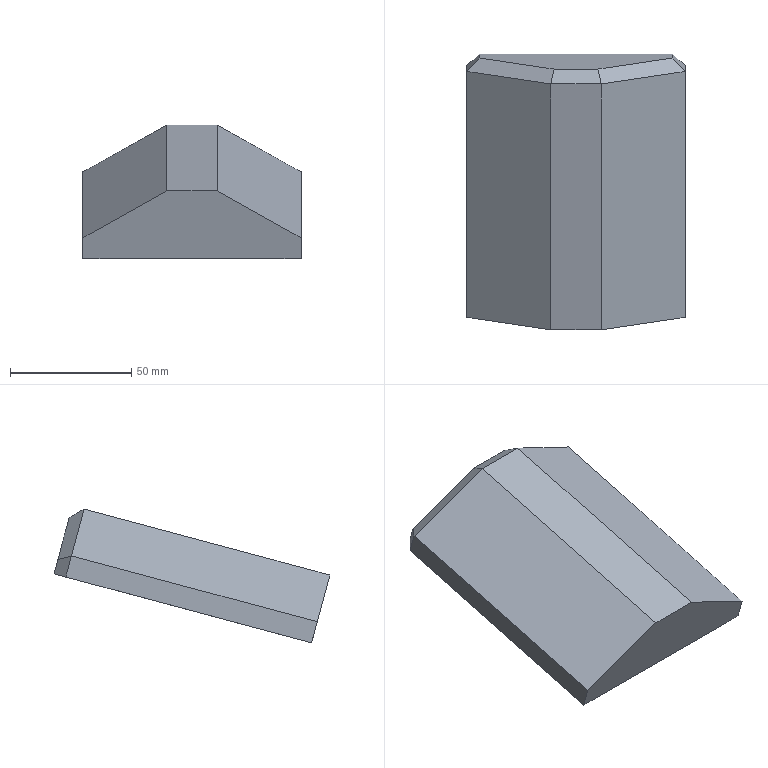Part | NX | features solid 2 | 1 solid | 13 faces | box 90 x 113.758 x 55.188 mm | volume 209622 mm3 | plane 13
STEP:
#1=CARTESIAN_POINT('',(-159.608,972.5,-215.013));
#2=VERTEX_POINT('',#1);
#3=CARTESIAN_POINT('',(-159.608,871.078,-242.189));
#4=VERTEX_POINT('',#3);
#5=CARTESIAN_POINT('',(-159.608,977.33,-213.718));
#6=DIRECTION('',(0.,-0.9659,-0.2588));
#7=VECTOR('',#6,1000.);
#8=LINE('',#5,#7);
#9=EDGE_CURVE('',#2,#4,#8,.T.);
#10=ORIENTED_EDGE('',*,*,#9,.F.);
#11=CARTESIAN_POINT('',(-180.392,972.5,-215.013));
#12=VERTEX_POINT('',#11);
#13=CARTESIAN_POINT('',(-180.392,972.5,-215.013));
#14=DIRECTION('',(-1.,-0.000000002,0.000000009));
#15=VECTOR('',#14,1000.);
#16=LINE('',#13,#15);
#17=EDGE_CURVE('',#2,#12,#16,.T.);
#18=ORIENTED_EDGE('',*,*,#17,.T.);
#19=CARTESIAN_POINT('',(-180.392,871.078,-242.189));
#20=VERTEX_POINT('',#19);
#21=CARTESIAN_POINT('',(-180.392,977.33,-213.718));
#22=DIRECTION('',(0.,-0.9659,-0.2588));
#23=VECTOR('',#22,1000.);
#24=LINE('',#21,#23);
#25=EDGE_CURVE('',#12,#20,#24,.T.);
#26=ORIENTED_EDGE('',*,*,#25,.T.);
#27=CARTESIAN_POINT('',(-180.392,871.078,-242.189));
#28=DIRECTION('',(1.,0.000000002,-0.000000009));
#29=VECTOR('',#28,1000.);
#30=LINE('',#27,#29);
#31=EDGE_CURVE('',#20,#4,#30,.T.);
#32=ORIENTED_EDGE('',*,*,#31,.T.);
#33=EDGE_LOOP('',(#10,#18,#26,#32));
#34=FACE_BOUND('',#33,.T.);
#35=CARTESIAN_POINT('',(-180.392,977.33,-213.718));
#36=DIRECTION('',(-0.00000001,0.2588,-0.9659));
#37=DIRECTION('',(0.,-0.9659,-0.2588));
#38=AXIS2_PLACEMENT_3D('',#35,#36,#37);
#39=PLANE('',#38);
#40=ADVANCED_FACE('',(#34),#39,.F.);
#41=CARTESIAN_POINT('',(-125.,977.672,-234.313));
#42=VERTEX_POINT('',#41);
#43=CARTESIAN_POINT('',(-125.,876.249,-261.489));
#44=VERTEX_POINT('',#43);
#45=CARTESIAN_POINT('',(-125.,982.501,-233.018));
#46=DIRECTION('',(0.,-0.9659,-0.2588));
#47=VECTOR('',#46,1000.);
#48=LINE('',#45,#47);
#49=EDGE_CURVE('',#42,#44,#48,.T.);
#50=ORIENTED_EDGE('',*,*,#49,.F.);
#51=CARTESIAN_POINT('',(-159.608,972.5,-215.013));
#52=DIRECTION('',(-0.866,-0.1294,0.483));
#53=VECTOR('',#52,1000.);
#54=LINE('',#51,#53);
#55=EDGE_CURVE('',#42,#2,#54,.T.);
#56=ORIENTED_EDGE('',*,*,#55,.T.);
#57=ORIENTED_EDGE('',*,*,#9,.T.);
#58=CARTESIAN_POINT('',(-126.699,875.996,-260.541));
#59=DIRECTION('',(0.866,0.1294,-0.483));
#60=VECTOR('',#59,1000.);
#61=LINE('',#58,#60);
#62=EDGE_CURVE('',#4,#44,#61,.T.);
#63=ORIENTED_EDGE('',*,*,#62,.T.);
#64=EDGE_LOOP('',(#50,#56,#57,#63));
#65=FACE_BOUND('',#64,.T.);
#66=CARTESIAN_POINT('',(-126.699,982.247,-232.071));
#67=DIRECTION('',(-0.5,0.2241,-0.8365));
#68=DIRECTION('',(0.8321,-0.1436,-0.5358));
#69=AXIS2_PLACEMENT_3D('',#66,#67,#68);
#70=PLANE('',#69);
#71=ADVANCED_FACE('',(#65),#70,.F.);
#72=CARTESIAN_POINT('',(-125.,980.006,-243.024));
#73=VERTEX_POINT('',#72);
#74=CARTESIAN_POINT('',(-125.,878.584,-270.2));
#75=VERTEX_POINT('',#74);
#76=CARTESIAN_POINT('',(-125.,984.836,-241.73));
#77=DIRECTION('',(0.,-0.9659,-0.2588));
#78=VECTOR('',#77,1000.);
#79=LINE('',#76,#78);
#80=EDGE_CURVE('',#73,#75,#79,.T.);
#81=ORIENTED_EDGE('',*,*,#80,.F.);
#82=CARTESIAN_POINT('',(-125.,977.672,-234.313));
#83=DIRECTION('',(0.000000016,-0.2588,0.9659));
#84=VECTOR('',#83,1000.);
#85=LINE('',#82,#84);
#86=EDGE_CURVE('',#73,#42,#85,.T.);
#87=ORIENTED_EDGE('',*,*,#86,.T.);
#88=ORIENTED_EDGE('',*,*,#49,.T.);
#89=CARTESIAN_POINT('',(-125.,876.249,-261.489));
#90=DIRECTION('',(-0.000000016,0.2588,-0.9659));
#91=VECTOR('',#90,1000.);
#92=LINE('',#89,#91);
#93=EDGE_CURVE('',#44,#75,#92,.T.);
#94=ORIENTED_EDGE('',*,*,#93,.T.);
#95=EDGE_LOOP('',(#81,#87,#88,#94));
#96=FACE_BOUND('',#95,.T.);
#97=CARTESIAN_POINT('',(-125.,982.501,-233.018));
#98=DIRECTION('',(-1.,-0.000000004,0.000000015));
#99=DIRECTION('',(-0.000000014,-0.2588,-0.9659));
#100=AXIS2_PLACEMENT_3D('',#97,#98,#99);
#101=PLANE('',#100);
#102=ADVANCED_FACE('',(#96),#101,.F.);
#103=CARTESIAN_POINT('',(-137.,984.836,-241.73));
#104=VERTEX_POINT('',#103);
#105=CARTESIAN_POINT('',(-130.,984.836,-241.73));
#106=VERTEX_POINT('',#105);
#107=CARTESIAN_POINT('',(-137.,984.836,-241.73));
#108=DIRECTION('',(1.,0.000000005,-0.000000017));
#109=VECTOR('',#108,1000.);
#110=LINE('',#107,#109);
#111=EDGE_CURVE('',#104,#106,#110,.T.);
#112=ORIENTED_EDGE('',*,*,#111,.T.);
#113=CARTESIAN_POINT('',(-130.,984.836,-241.73));
#114=DIRECTION('',(0.7071,-0.683,-0.183));
#115=VECTOR('',#114,1000.);
#116=LINE('',#113,#115);
#117=EDGE_CURVE('',#106,#73,#116,.T.);
#118=ORIENTED_EDGE('',*,*,#117,.T.);
#119=ORIENTED_EDGE('',*,*,#80,.T.);
#120=CARTESIAN_POINT('',(-137.,878.584,-270.2));
#121=VERTEX_POINT('',#120);
#122=CARTESIAN_POINT('',(-137.,878.584,-270.2));
#123=DIRECTION('',(1.,0.000000005,-0.000000017));
#124=VECTOR('',#123,1000.);
#125=LINE('',#122,#124);
#126=EDGE_CURVE('',#121,#75,#125,.T.);
#127=ORIENTED_EDGE('',*,*,#126,.F.);
#128=CARTESIAN_POINT('',(-203.,878.584,-270.2));
#129=VERTEX_POINT('',#128);
#130=CARTESIAN_POINT('',(-203.,878.584,-270.2));
#131=DIRECTION('',(1.,0.,0.000000001));
#132=VECTOR('',#131,1000.);
#133=LINE('',#130,#132);
#134=EDGE_CURVE('',#129,#121,#133,.T.);
#135=ORIENTED_EDGE('',*,*,#134,.F.);
#136=CARTESIAN_POINT('',(-215.,878.584,-270.2));
#137=VERTEX_POINT('',#136);
#138=CARTESIAN_POINT('',(-208.,878.584,-270.2));
#139=DIRECTION('',(-1.,-0.000000005,0.000000017));
#140=VECTOR('',#139,1000.);
#141=LINE('',#138,#140);
#142=EDGE_CURVE('',#137,#129,#141,.F.);
#143=ORIENTED_EDGE('',*,*,#142,.F.);
#144=CARTESIAN_POINT('',(-215.,980.006,-243.024));
#145=VERTEX_POINT('',#144);
#146=CARTESIAN_POINT('',(-215.,984.836,-241.73));
#147=DIRECTION('',(0.,-0.9659,-0.2588));
#148=VECTOR('',#147,1000.);
#149=LINE('',#146,#148);
#150=EDGE_CURVE('',#145,#137,#149,.T.);
#151=ORIENTED_EDGE('',*,*,#150,.F.);
#152=CARTESIAN_POINT('',(-210.,984.836,-241.73));
#153=VERTEX_POINT('',#152);
#154=CARTESIAN_POINT('',(-215.,980.006,-243.024));
#155=DIRECTION('',(-0.7071,-0.683,-0.183));
#156=VECTOR('',#155,1000.);
#157=LINE('',#154,#156);
#158=EDGE_CURVE('',#145,#153,#157,.F.);
#159=ORIENTED_EDGE('',*,*,#158,.T.);
#160=CARTESIAN_POINT('',(-203.,984.836,-241.73));
#161=VERTEX_POINT('',#160);
#162=CARTESIAN_POINT('',(-208.,984.836,-241.73));
#163=DIRECTION('',(-1.,-0.000000005,0.000000017));
#164=VECTOR('',#163,1000.);
#165=LINE('',#162,#164);
#166=EDGE_CURVE('',#153,#161,#165,.F.);
#167=ORIENTED_EDGE('',*,*,#166,.T.);
#168=CARTESIAN_POINT('',(-203.,984.836,-241.73));
#169=DIRECTION('',(1.,0.,0.000000001));
#170=VECTOR('',#169,1000.);
#171=LINE('',#168,#170);
#172=EDGE_CURVE('',#161,#104,#171,.T.);
#173=ORIENTED_EDGE('',*,*,#172,.T.);
#174=EDGE_LOOP('',(#112,#118,#119,#127,#135,#143,#151,#159,#167,#173));
#175=FACE_BOUND('',#174,.T.);
#176=CARTESIAN_POINT('',(-208.,984.836,-241.73));
#177=DIRECTION('',(0.000000018,-0.2588,0.9659));
#178=DIRECTION('',(0.,0.9659,0.2588));
#179=AXIS2_PLACEMENT_3D('',#176,#177,#178);
#180=PLANE('',#179);
#181=ADVANCED_FACE('',(#175),#180,.F.);
#182=CARTESIAN_POINT('',(-215.,977.672,-234.313));
#183=VERTEX_POINT('',#182);
#184=CARTESIAN_POINT('',(-215.,876.249,-261.489));
#185=VERTEX_POINT('',#184);
#186=CARTESIAN_POINT('',(-215.,982.501,-233.018));
#187=DIRECTION('',(0.,-0.9659,-0.2588));
#188=VECTOR('',#187,1000.);
#189=LINE('',#186,#188);
#190=EDGE_CURVE('',#183,#185,#189,.T.);
#191=ORIENTED_EDGE('',*,*,#190,.F.);
#192=CARTESIAN_POINT('',(-215.,977.672,-234.313));
#193=DIRECTION('',(-0.000000016,0.2588,-0.9659));
#194=VECTOR('',#193,1000.);
#195=LINE('',#192,#194);
#196=EDGE_CURVE('',#183,#145,#195,.T.);
#197=ORIENTED_EDGE('',*,*,#196,.T.);
#198=ORIENTED_EDGE('',*,*,#150,.T.);
#199=CARTESIAN_POINT('',(-215.,876.249,-261.489));
#200=DIRECTION('',(-0.000000016,0.2588,-0.9659));
#201=VECTOR('',#200,1000.);
#202=LINE('',#199,#201);
#203=EDGE_CURVE('',#185,#137,#202,.T.);
#204=ORIENTED_EDGE('',*,*,#203,.F.);
#205=EDGE_LOOP('',(#191,#197,#198,#204));
#206=FACE_BOUND('',#205,.T.);
#207=CARTESIAN_POINT('',(-215.,982.501,-233.018));
#208=DIRECTION('',(-1.,-0.000000004,0.000000015));
#209=DIRECTION('',(-0.000000014,-0.2588,-0.9659));
#210=AXIS2_PLACEMENT_3D('',#207,#208,#209);
#211=PLANE('',#210);
#212=ADVANCED_FACE('',(#206),#211,.T.);
#213=ORIENTED_EDGE('',*,*,#25,.F.);
#214=CARTESIAN_POINT('',(-180.392,972.5,-215.013));
#215=DIRECTION('',(-0.866,0.1294,-0.483));
#216=VECTOR('',#215,1000.);
#217=LINE('',#214,#216);
#218=EDGE_CURVE('',#12,#183,#217,.T.);
#219=ORIENTED_EDGE('',*,*,#218,.T.);
#220=ORIENTED_EDGE('',*,*,#190,.T.);
#221=CARTESIAN_POINT('',(-180.392,871.078,-242.189));
#222=DIRECTION('',(-0.866,0.1294,-0.483));
#223=VECTOR('',#222,1000.);
#224=LINE('',#221,#223);
#225=EDGE_CURVE('',#20,#185,#224,.T.);
#226=ORIENTED_EDGE('',*,*,#225,.F.);
#227=EDGE_LOOP('',(#213,#219,#220,#226));
#228=FACE_BOUND('',#227,.T.);
#229=CARTESIAN_POINT('',(-180.392,977.33,-213.718));
#230=DIRECTION('',(-0.5,-0.2241,0.8365));
#231=DIRECTION('',(-0.8321,-0.1436,-0.5358));
#232=AXIS2_PLACEMENT_3D('',#229,#230,#231);
#233=PLANE('',#232);
#234=ADVANCED_FACE('',(#228),#233,.T.);
#235=CARTESIAN_POINT('',(-160.947,978.624,-218.548));
#236=VERTEX_POINT('',#235);
#237=CARTESIAN_POINT('',(-130.,983.248,-235.807));
#238=VERTEX_POINT('',#237);
#239=CARTESIAN_POINT('',(-127.5,983.622,-237.201));
#240=DIRECTION('',(0.866,0.1294,-0.483));
#241=VECTOR('',#240,1000.);
#242=LINE('',#239,#241);
#243=EDGE_CURVE('',#236,#238,#242,.T.);
#244=ORIENTED_EDGE('',*,*,#243,.T.);
#245=CARTESIAN_POINT('',(-130.,984.836,-241.73));
#246=DIRECTION('',(-0.000000016,0.2588,-0.9659));
#247=VECTOR('',#246,1000.);
#248=LINE('',#245,#247);
#249=EDGE_CURVE('',#238,#106,#248,.T.);
#250=ORIENTED_EDGE('',*,*,#249,.T.);
#251=ORIENTED_EDGE('',*,*,#111,.F.);
#252=ORIENTED_EDGE('',*,*,#172,.F.);
#253=ORIENTED_EDGE('',*,*,#166,.F.);
#254=CARTESIAN_POINT('',(-210.,983.248,-235.807));
#255=VERTEX_POINT('',#254);
#256=CARTESIAN_POINT('',(-210.,977.33,-213.718));
#257=DIRECTION('',(0.000000016,-0.2588,0.9659));
#258=VECTOR('',#257,1000.);
#259=LINE('',#256,#258);
#260=EDGE_CURVE('',#153,#255,#259,.T.);
#261=ORIENTED_EDGE('',*,*,#260,.T.);
#262=CARTESIAN_POINT('',(-179.053,978.624,-218.548));
#263=VERTEX_POINT('',#262);
#264=CARTESIAN_POINT('',(-136.348,972.243,-194.733));
#265=DIRECTION('',(0.866,-0.1294,0.483));
#266=VECTOR('',#265,1000.);
#267=LINE('',#264,#266);
#268=EDGE_CURVE('',#255,#263,#267,.T.);
#269=ORIENTED_EDGE('',*,*,#268,.T.);
#270=CARTESIAN_POINT('',(-159.608,978.624,-218.548));
#271=DIRECTION('',(1.,0.000000002,-0.000000009));
#272=VECTOR('',#271,1000.);
#273=LINE('',#270,#272);
#274=EDGE_CURVE('',#263,#236,#273,.T.);
#275=ORIENTED_EDGE('',*,*,#274,.T.);
#276=EDGE_LOOP('',(#244,#250,#251,#252,#253,#261,#269,#275));
#277=FACE_BOUND('',#276,.T.);
#278=CARTESIAN_POINT('',(-125.,977.33,-213.718));
#279=DIRECTION('',(0.,0.9659,0.2588));
#280=DIRECTION('',(0.,0.2588,-0.9659));
#281=AXIS2_PLACEMENT_3D('',#278,#279,#280);
#282=PLANE('',#281);
#283=ADVANCED_FACE('',(#277),#282,.T.);
#284=ORIENTED_EDGE('',*,*,#31,.F.);
#285=ORIENTED_EDGE('',*,*,#225,.T.);
#286=ORIENTED_EDGE('',*,*,#203,.T.);
#287=ORIENTED_EDGE('',*,*,#142,.T.);
#288=ORIENTED_EDGE('',*,*,#134,.T.);
#289=ORIENTED_EDGE('',*,*,#126,.T.);
#290=ORIENTED_EDGE('',*,*,#93,.F.);
#291=ORIENTED_EDGE('',*,*,#62,.F.);
#292=EDGE_LOOP('',(#284,#285,#286,#287,#288,#289,#290,#291));
#293=FACE_BOUND('',#292,.T.);
#294=CARTESIAN_POINT('',(-125.,871.078,-242.189));
#295=DIRECTION('',(0.,0.9659,0.2588));
#296=DIRECTION('',(0.,0.2588,-0.9659));
#297=AXIS2_PLACEMENT_3D('',#294,#295,#296);
#298=PLANE('',#297);
#299=ADVANCED_FACE('',(#293),#298,.F.);
#300=ORIENTED_EDGE('',*,*,#158,.F.);
#301=ORIENTED_EDGE('',*,*,#196,.F.);
#302=CARTESIAN_POINT('',(-215.,977.672,-234.313));
#303=DIRECTION('',(0.6547,0.7302,-0.1956));
#304=VECTOR('',#303,1000.);
#305=LINE('',#302,#304);
#306=EDGE_CURVE('',#255,#183,#305,.F.);
#307=ORIENTED_EDGE('',*,*,#306,.F.);
#308=ORIENTED_EDGE('',*,*,#260,.F.);
#309=EDGE_LOOP('',(#300,#301,#307,#308));
#310=FACE_BOUND('',#309,.T.);
#311=CARTESIAN_POINT('',(-215.,977.672,-234.313));
#312=DIRECTION('',(0.7071,-0.683,-0.183));
#313=DIRECTION('',(0.6715,0.7297,-0.1287));
#314=AXIS2_PLACEMENT_3D('',#311,#312,#313);
#315=PLANE('',#314);
#316=ADVANCED_FACE('',(#310),#315,.F.);
#317=ORIENTED_EDGE('',*,*,#306,.T.);
#318=ORIENTED_EDGE('',*,*,#218,.F.);
#319=CARTESIAN_POINT('',(-180.392,972.5,-215.013));
#320=DIRECTION('',(-0.1862,-0.8509,0.4913));
#321=VECTOR('',#320,1000.);
#322=LINE('',#319,#321);
#323=EDGE_CURVE('',#263,#12,#322,.T.);
#324=ORIENTED_EDGE('',*,*,#323,.F.);
#325=ORIENTED_EDGE('',*,*,#268,.F.);
#326=EDGE_LOOP('',(#317,#318,#324,#325));
#327=FACE_BOUND('',#326,.T.);
#328=CARTESIAN_POINT('',(-180.392,972.5,-215.013));
#329=DIRECTION('',(0.3536,-0.5245,-0.7745));
#330=DIRECTION('',(0.,-0.828,0.5607));
#331=AXIS2_PLACEMENT_3D('',#328,#329,#330);
#332=PLANE('',#331);
#333=ADVANCED_FACE('',(#327),#332,.F.);
#334=ORIENTED_EDGE('',*,*,#323,.T.);
#335=ORIENTED_EDGE('',*,*,#17,.F.);
#336=CARTESIAN_POINT('',(-159.702,972.93,-215.261));
#337=DIRECTION('',(-0.1862,0.8509,-0.4913));
#338=VECTOR('',#337,1000.);
#339=LINE('',#336,#338);
#340=EDGE_CURVE('',#236,#2,#339,.F.);
#341=ORIENTED_EDGE('',*,*,#340,.F.);
#342=ORIENTED_EDGE('',*,*,#274,.F.);
#343=EDGE_LOOP('',(#334,#335,#341,#342));
#344=FACE_BOUND('',#343,.T.);
#345=CARTESIAN_POINT('',(-125.,978.624,-218.548));
#346=DIRECTION('',(0.000000007,0.5,0.866));
#347=DIRECTION('',(0.,0.866,-0.5));
#348=AXIS2_PLACEMENT_3D('',#345,#346,#347);
#349=PLANE('',#348);
#350=ADVANCED_FACE('',(#344),#349,.T.);
#351=ORIENTED_EDGE('',*,*,#340,.T.);
#352=ORIENTED_EDGE('',*,*,#55,.F.);
#353=CARTESIAN_POINT('',(-131.758,985.209,-236.332));
#354=DIRECTION('',(-0.6547,0.7302,-0.1956));
#355=VECTOR('',#354,1000.);
#356=LINE('',#353,#355);
#357=EDGE_CURVE('',#238,#42,#356,.F.);
#358=ORIENTED_EDGE('',*,*,#357,.F.);
#359=ORIENTED_EDGE('',*,*,#243,.F.);
#360=EDGE_LOOP('',(#351,#352,#358,#359));
#361=FACE_BOUND('',#360,.T.);
#362=CARTESIAN_POINT('',(-136.152,982.329,-232.376));
#363=DIRECTION('',(0.3536,0.5245,0.7745));
#364=DIRECTION('',(0.,0.828,-0.5607));
#365=AXIS2_PLACEMENT_3D('',#362,#363,#364);
#366=PLANE('',#365);
#367=ADVANCED_FACE('',(#361),#366,.T.);
#368=ORIENTED_EDGE('',*,*,#357,.T.);
#369=ORIENTED_EDGE('',*,*,#86,.F.);
#370=ORIENTED_EDGE('',*,*,#117,.F.);
#371=ORIENTED_EDGE('',*,*,#249,.F.);
#372=EDGE_LOOP('',(#368,#369,#370,#371));
#373=FACE_BOUND('',#372,.T.);
#374=CARTESIAN_POINT('',(-130.,977.33,-213.718));
#375=DIRECTION('',(0.7071,0.683,0.183));
#376=DIRECTION('',(-0.6715,0.7297,-0.1287));
#377=AXIS2_PLACEMENT_3D('',#374,#375,#376);
#378=PLANE('',#377);
#379=ADVANCED_FACE('',(#373),#378,.T.);
#380=CLOSED_SHELL('',(#40,#71,#102,#181,#212,#234,#283,#299,#316,#333,#350,#367,#379));
#381=MANIFOLD_SOLID_BREP('',#380);
#382=(LENGTH_UNIT()NAMED_UNIT(*)SI_UNIT(.MILLI.,.METRE.));
#383=UNCERTAINTY_MEASURE_WITH_UNIT(LENGTH_MEASURE(0.00001),#382,'','');
#384=(NAMED_UNIT(*)PLANE_ANGLE_UNIT()SI_UNIT($,.RADIAN.));
#385=(NAMED_UNIT(*)SI_UNIT($,.STERADIAN.)SOLID_ANGLE_UNIT());
#386=(GEOMETRIC_REPRESENTATION_CONTEXT(3)GLOBAL_UNCERTAINTY_ASSIGNED_CONTEXT((#383))GLOBAL_UNIT_ASSIGNED_CONTEXT((#382,#384,#385))REPRESENTATION_CONTEXT('',''));
#387=ADVANCED_BREP_SHAPE_REPRESENTATION('',(#381),#386);